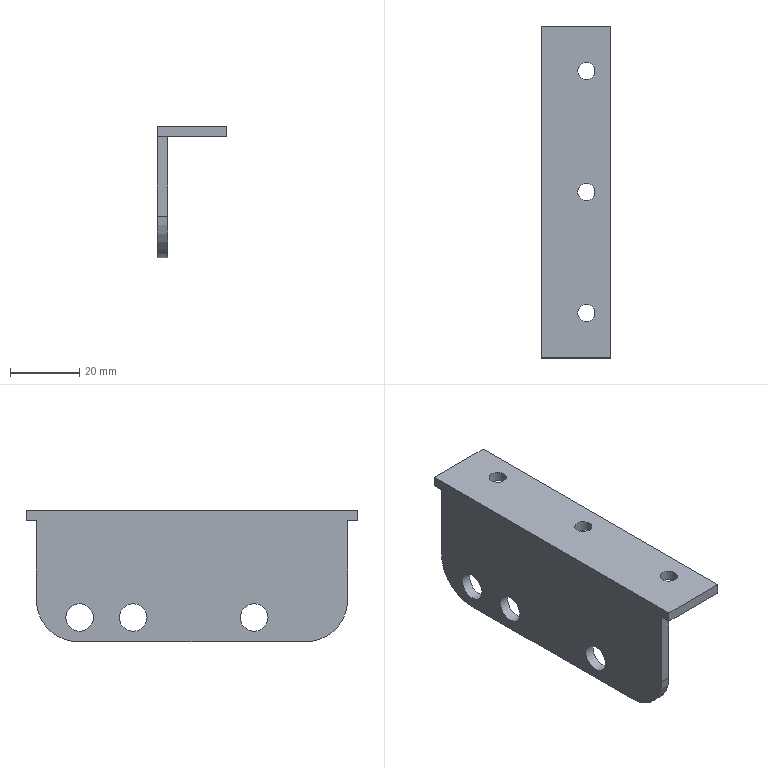Part | STEP file | 1-43.8 | 1 solid | 18 faces | box 20 x 96 x 38 mm | volume 14395 mm3 | plane 10 | cylinder 8 | commonest cylinder face diameters 5 x3 8 x3 24 x2
STEP:
#1=CARTESIAN_POINT('',(0.,0.,0.));
#2=DIRECTION('',(0.,0.,1.));
#3=DIRECTION('',(1.,0.,0.));
#4=AXIS2_PLACEMENT_3D('',#1,#2,#3);
#5=CARTESIAN_POINT('',(10.,-48.,3.));
#6=VERTEX_POINT('',#5);
#7=CARTESIAN_POINT('',(10.,48.,3.));
#8=VERTEX_POINT('',#7);
#9=CARTESIAN_POINT('',(10.,-48.,3.));
#10=DIRECTION('',(0.,1.,0.));
#11=VECTOR('',#10,1.);
#12=LINE('',#9,#11);
#13=CARTESIAN_POINT('',(-38.,0.,3.));
#14=DIRECTION('',(0.,0.,1.));
#15=DIRECTION('',(0.,1.,0.));
#16=AXIS2_PLACEMENT_3D('',#13,#14,#15);
#17=PLANE('',#16);
#18=CARTESIAN_POINT('',(-48.,-48.));
#19=DIRECTION('',(1.,0.));
#20=VECTOR('',#19,1.);
#21=LINE('',#18,#20);
#22=(GEOMETRIC_REPRESENTATION_CONTEXT(2)PARAMETRIC_REPRESENTATION_CONTEXT()REPRESENTATION_CONTEXT('',''));
#23=DEFINITIONAL_REPRESENTATION('',(#21),#22);
#24=PCURVE('',#17,#23);
#25=CARTESIAN_POINT('',(10.,0.,1.5));
#26=DIRECTION('',(1.,0.,0.));
#27=DIRECTION('',(0.,1.,0.));
#28=AXIS2_PLACEMENT_3D('',#25,#26,#27);
#29=PLANE('',#28);
#30=CARTESIAN_POINT('',(-48.,1.5));
#31=DIRECTION('',(1.,0.));
#32=VECTOR('',#31,1.);
#33=LINE('',#30,#32);
#34=(GEOMETRIC_REPRESENTATION_CONTEXT(2)PARAMETRIC_REPRESENTATION_CONTEXT()REPRESENTATION_CONTEXT('',''));
#35=DEFINITIONAL_REPRESENTATION('',(#33),#34);
#36=PCURVE('',#29,#35);
#37=SURFACE_CURVE('',#12,(#24,#36),.PCURVE_S1.);
#38=EDGE_CURVE('',#6,#8,#37,.T.);
#39=ORIENTED_EDGE('',*,*,#38,.T.);
#40=CARTESIAN_POINT('',(-10.,48.,3.));
#41=VERTEX_POINT('',#40);
#42=CARTESIAN_POINT('',(10.,48.,3.));
#43=DIRECTION('',(-1.,0.,0.));
#44=VECTOR('',#43,1.);
#45=LINE('',#42,#44);
#46=CARTESIAN_POINT('',(48.,-48.));
#47=DIRECTION('',(0.,1.));
#48=VECTOR('',#47,1.);
#49=LINE('',#46,#48);
#50=(GEOMETRIC_REPRESENTATION_CONTEXT(2)PARAMETRIC_REPRESENTATION_CONTEXT()REPRESENTATION_CONTEXT('',''));
#51=DEFINITIONAL_REPRESENTATION('',(#49),#50);
#52=PCURVE('',#17,#51);
#53=CARTESIAN_POINT('',(0.,48.,1.5));
#54=DIRECTION('',(0.,1.,0.));
#55=DIRECTION('',(-1.,0.,0.));
#56=AXIS2_PLACEMENT_3D('',#53,#54,#55);
#57=PLANE('',#56);
#58=CARTESIAN_POINT('',(-10.,1.5));
#59=DIRECTION('',(1.,0.));
#60=VECTOR('',#59,1.);
#61=LINE('',#58,#60);
#62=(GEOMETRIC_REPRESENTATION_CONTEXT(2)PARAMETRIC_REPRESENTATION_CONTEXT()REPRESENTATION_CONTEXT('',''));
#63=DEFINITIONAL_REPRESENTATION('',(#61),#62);
#64=PCURVE('',#57,#63);
#65=SURFACE_CURVE('',#45,(#52,#64),.PCURVE_S1.);
#66=EDGE_CURVE('',#8,#41,#65,.T.);
#67=ORIENTED_EDGE('',*,*,#66,.T.);
#68=CARTESIAN_POINT('',(-10.,-48.,3.));
#69=VERTEX_POINT('',#68);
#70=CARTESIAN_POINT('',(-10.,48.,3.));
#71=DIRECTION('',(0.,-1.,0.));
#72=VECTOR('',#71,1.);
#73=LINE('',#70,#72);
#74=CARTESIAN_POINT('',(48.,-28.));
#75=DIRECTION('',(-1.,0.));
#76=VECTOR('',#75,1.);
#77=LINE('',#74,#76);
#78=(GEOMETRIC_REPRESENTATION_CONTEXT(2)PARAMETRIC_REPRESENTATION_CONTEXT()REPRESENTATION_CONTEXT('',''));
#79=DEFINITIONAL_REPRESENTATION('',(#77),#78);
#80=PCURVE('',#17,#79);
#81=CARTESIAN_POINT('',(-10.,0.,10.));
#82=DIRECTION('',(-1.,0.,0.));
#83=DIRECTION('',(0.,-1.,0.));
#84=AXIS2_PLACEMENT_3D('',#81,#82,#83);
#85=PLANE('',#84);
#86=CARTESIAN_POINT('',(-48.,-7.));
#87=DIRECTION('',(1.,0.));
#88=VECTOR('',#87,1.);
#89=LINE('',#86,#88);
#90=(GEOMETRIC_REPRESENTATION_CONTEXT(2)PARAMETRIC_REPRESENTATION_CONTEXT()REPRESENTATION_CONTEXT('',''));
#91=DEFINITIONAL_REPRESENTATION('',(#89),#90);
#92=PCURVE('',#85,#91);
#93=SURFACE_CURVE('',#73,(#80,#92),.PCURVE_S1.);
#94=EDGE_CURVE('',#41,#69,#93,.T.);
#95=ORIENTED_EDGE('',*,*,#94,.T.);
#96=CARTESIAN_POINT('',(-10.,-48.,3.));
#97=DIRECTION('',(1.,0.,0.));
#98=VECTOR('',#97,1.);
#99=LINE('',#96,#98);
#100=CARTESIAN_POINT('',(-48.,-28.));
#101=DIRECTION('',(0.,-1.));
#102=VECTOR('',#101,1.);
#103=LINE('',#100,#102);
#104=(GEOMETRIC_REPRESENTATION_CONTEXT(2)PARAMETRIC_REPRESENTATION_CONTEXT()REPRESENTATION_CONTEXT('',''));
#105=DEFINITIONAL_REPRESENTATION('',(#103),#104);
#106=PCURVE('',#17,#105);
#107=CARTESIAN_POINT('',(0.,-48.,1.5));
#108=DIRECTION('',(0.,-1.,0.));
#109=DIRECTION('',(1.,0.,0.));
#110=AXIS2_PLACEMENT_3D('',#107,#108,#109);
#111=PLANE('',#110);
#112=CARTESIAN_POINT('',(-10.,1.5));
#113=DIRECTION('',(1.,0.));
#114=VECTOR('',#113,1.);
#115=LINE('',#112,#114);
#116=(GEOMETRIC_REPRESENTATION_CONTEXT(2)PARAMETRIC_REPRESENTATION_CONTEXT()REPRESENTATION_CONTEXT('',''));
#117=DEFINITIONAL_REPRESENTATION('',(#115),#116);
#118=PCURVE('',#111,#117);
#119=SURFACE_CURVE('',#99,(#106,#118),.PCURVE_S1.);
#120=EDGE_CURVE('',#69,#6,#119,.T.);
#121=ORIENTED_EDGE('',*,*,#120,.T.);
#122=EDGE_LOOP('',(#39,#67,#95,#121));
#123=FACE_BOUND('',#122,.T.);
#124=CARTESIAN_POINT('',(3.,2.5,3.));
#125=VERTEX_POINT('',#124);
#126=CARTESIAN_POINT('',(3.,0.,3.));
#127=DIRECTION('',(0.,0.,-1.));
#128=DIRECTION('',(0.,1.,0.));
#129=AXIS2_PLACEMENT_3D('',#126,#127,#128);
#130=CIRCLE('',#129,2.5);
#131=CARTESIAN_POINT('',(2.5,-41.));
#132=CARTESIAN_POINT('',(2.5,-45.33));
#133=CARTESIAN_POINT('',(-1.25,-43.165));
#134=CARTESIAN_POINT('',(-5.,-41.));
#135=CARTESIAN_POINT('',(-1.25,-38.835));
#136=CARTESIAN_POINT('',(2.5,-36.67));
#137=CARTESIAN_POINT('',(2.5,-41.));
#138=(BOUNDED_CURVE()B_SPLINE_CURVE(2,(#131,#132,#133,#134,#135,#136,#137),.UNSPECIFIED.,.T.,.F.)B_SPLINE_CURVE_WITH_KNOTS((1,2,2,2,2,1),(-2.094,0.,2.094,4.189,6.283,8.378),.UNSPECIFIED.)CURVE()GEOMETRIC_REPRESENTATION_ITEM()RATIONAL_B_SPLINE_CURVE((1.,0.5,1.,0.5,1.,0.5,1.))REPRESENTATION_ITEM(''));
#139=(GEOMETRIC_REPRESENTATION_CONTEXT(2)PARAMETRIC_REPRESENTATION_CONTEXT()REPRESENTATION_CONTEXT('',''));
#140=DEFINITIONAL_REPRESENTATION('',(#138),#139);
#141=PCURVE('',#17,#140);
#142=CARTESIAN_POINT('',(3.,0.,0.));
#143=DIRECTION('',(0.,0.,1.));
#144=DIRECTION('',(0.,1.,0.));
#145=AXIS2_PLACEMENT_3D('',#142,#143,#144);
#146=CYLINDRICAL_SURFACE('',#145,2.5);
#147=CARTESIAN_POINT('',(6.283,3.));
#148=DIRECTION('',(-1.,0.));
#149=VECTOR('',#148,1.);
#150=LINE('',#147,#149);
#151=(GEOMETRIC_REPRESENTATION_CONTEXT(2)PARAMETRIC_REPRESENTATION_CONTEXT()REPRESENTATION_CONTEXT('',''));
#152=DEFINITIONAL_REPRESENTATION('',(#150),#151);
#153=PCURVE('',#146,#152);
#154=SURFACE_CURVE('',#130,(#141,#153),.PCURVE_S1.);
#155=EDGE_CURVE('',#125,#125,#154,.T.);
#156=ORIENTED_EDGE('',*,*,#155,.T.);
#157=EDGE_LOOP('',(#156));
#158=FACE_BOUND('',#157,.T.);
#159=CARTESIAN_POINT('',(3.,-32.5,3.));
#160=VERTEX_POINT('',#159);
#161=CARTESIAN_POINT('',(3.,-35.,3.));
#162=DIRECTION('',(0.,0.,-1.));
#163=DIRECTION('',(0.,1.,0.));
#164=AXIS2_PLACEMENT_3D('',#161,#162,#163);
#165=CIRCLE('',#164,2.5);
#166=CARTESIAN_POINT('',(-32.5,-41.));
#167=CARTESIAN_POINT('',(-32.5,-45.33));
#168=CARTESIAN_POINT('',(-36.25,-43.165));
#169=CARTESIAN_POINT('',(-40.,-41.));
#170=CARTESIAN_POINT('',(-36.25,-38.835));
#171=CARTESIAN_POINT('',(-32.5,-36.67));
#172=CARTESIAN_POINT('',(-32.5,-41.));
#173=(BOUNDED_CURVE()B_SPLINE_CURVE(2,(#166,#167,#168,#169,#170,#171,#172),.UNSPECIFIED.,.T.,.F.)B_SPLINE_CURVE_WITH_KNOTS((1,2,2,2,2,1),(-2.094,0.,2.094,4.189,6.283,8.378),.UNSPECIFIED.)CURVE()GEOMETRIC_REPRESENTATION_ITEM()RATIONAL_B_SPLINE_CURVE((1.,0.5,1.,0.5,1.,0.5,1.))REPRESENTATION_ITEM(''));
#174=(GEOMETRIC_REPRESENTATION_CONTEXT(2)PARAMETRIC_REPRESENTATION_CONTEXT()REPRESENTATION_CONTEXT('',''));
#175=DEFINITIONAL_REPRESENTATION('',(#173),#174);
#176=PCURVE('',#17,#175);
#177=CARTESIAN_POINT('',(3.,-35.,0.));
#178=DIRECTION('',(0.,0.,1.));
#179=DIRECTION('',(0.,1.,0.));
#180=AXIS2_PLACEMENT_3D('',#177,#178,#179);
#181=CYLINDRICAL_SURFACE('',#180,2.5);
#182=CARTESIAN_POINT('',(6.283,3.));
#183=DIRECTION('',(-1.,0.));
#184=VECTOR('',#183,1.);
#185=LINE('',#182,#184);
#186=(GEOMETRIC_REPRESENTATION_CONTEXT(2)PARAMETRIC_REPRESENTATION_CONTEXT()REPRESENTATION_CONTEXT('',''));
#187=DEFINITIONAL_REPRESENTATION('',(#185),#186);
#188=PCURVE('',#181,#187);
#189=SURFACE_CURVE('',#165,(#176,#188),.PCURVE_S1.);
#190=EDGE_CURVE('',#160,#160,#189,.T.);
#191=ORIENTED_EDGE('',*,*,#190,.T.);
#192=EDGE_LOOP('',(#191));
#193=FACE_BOUND('',#192,.T.);
#194=CARTESIAN_POINT('',(3.,37.5,3.));
#195=VERTEX_POINT('',#194);
#196=CARTESIAN_POINT('',(3.,35.,3.));
#197=DIRECTION('',(0.,0.,-1.));
#198=DIRECTION('',(0.,1.,0.));
#199=AXIS2_PLACEMENT_3D('',#196,#197,#198);
#200=CIRCLE('',#199,2.5);
#201=CARTESIAN_POINT('',(37.5,-41.));
#202=CARTESIAN_POINT('',(37.5,-45.33));
#203=CARTESIAN_POINT('',(33.75,-43.165));
#204=CARTESIAN_POINT('',(30.,-41.));
#205=CARTESIAN_POINT('',(33.75,-38.835));
#206=CARTESIAN_POINT('',(37.5,-36.67));
#207=CARTESIAN_POINT('',(37.5,-41.));
#208=(BOUNDED_CURVE()B_SPLINE_CURVE(2,(#201,#202,#203,#204,#205,#206,#207),.UNSPECIFIED.,.T.,.F.)B_SPLINE_CURVE_WITH_KNOTS((1,2,2,2,2,1),(-2.094,0.,2.094,4.189,6.283,8.378),.UNSPECIFIED.)CURVE()GEOMETRIC_REPRESENTATION_ITEM()RATIONAL_B_SPLINE_CURVE((1.,0.5,1.,0.5,1.,0.5,1.))REPRESENTATION_ITEM(''));
#209=(GEOMETRIC_REPRESENTATION_CONTEXT(2)PARAMETRIC_REPRESENTATION_CONTEXT()REPRESENTATION_CONTEXT('',''));
#210=DEFINITIONAL_REPRESENTATION('',(#208),#209);
#211=PCURVE('',#17,#210);
#212=CARTESIAN_POINT('',(3.,35.,0.));
#213=DIRECTION('',(0.,0.,1.));
#214=DIRECTION('',(0.,1.,0.));
#215=AXIS2_PLACEMENT_3D('',#212,#213,#214);
#216=CYLINDRICAL_SURFACE('',#215,2.5);
#217=CARTESIAN_POINT('',(6.283,3.));
#218=DIRECTION('',(-1.,0.));
#219=VECTOR('',#218,1.);
#220=LINE('',#217,#219);
#221=(GEOMETRIC_REPRESENTATION_CONTEXT(2)PARAMETRIC_REPRESENTATION_CONTEXT()REPRESENTATION_CONTEXT('',''));
#222=DEFINITIONAL_REPRESENTATION('',(#220),#221);
#223=PCURVE('',#216,#222);
#224=SURFACE_CURVE('',#200,(#211,#223),.PCURVE_S1.);
#225=EDGE_CURVE('',#195,#195,#224,.T.);
#226=ORIENTED_EDGE('',*,*,#225,.T.);
#227=EDGE_LOOP('',(#226));
#228=FACE_BOUND('',#227,.T.);
#229=ADVANCED_FACE('',(#123,#158,#193,#228),#17,.T.);
#230=CARTESIAN_POINT('',(10.,-48.,0.));
#231=VERTEX_POINT('',#230);
#232=CARTESIAN_POINT('',(10.,48.,0.));
#233=VERTEX_POINT('',#232);
#234=CARTESIAN_POINT('',(10.,-48.,0.));
#235=DIRECTION('',(0.,1.,0.));
#236=VECTOR('',#235,1.);
#237=LINE('',#234,#236);
#238=CARTESIAN_POINT('',(-48.,-1.5));
#239=DIRECTION('',(1.,0.));
#240=VECTOR('',#239,1.);
#241=LINE('',#238,#240);
#242=(GEOMETRIC_REPRESENTATION_CONTEXT(2)PARAMETRIC_REPRESENTATION_CONTEXT()REPRESENTATION_CONTEXT('',''));
#243=DEFINITIONAL_REPRESENTATION('',(#241),#242);
#244=PCURVE('',#29,#243);
#245=CARTESIAN_POINT('',(-38.,0.,0.));
#246=DIRECTION('',(0.,0.,1.));
#247=DIRECTION('',(0.,1.,0.));
#248=AXIS2_PLACEMENT_3D('',#245,#246,#247);
#249=PLANE('',#248);
#250=CARTESIAN_POINT('',(-48.,-48.));
#251=DIRECTION('',(1.,0.));
#252=VECTOR('',#251,1.);
#253=LINE('',#250,#252);
#254=(GEOMETRIC_REPRESENTATION_CONTEXT(2)PARAMETRIC_REPRESENTATION_CONTEXT()REPRESENTATION_CONTEXT('',''));
#255=DEFINITIONAL_REPRESENTATION('',(#253),#254);
#256=PCURVE('',#249,#255);
#257=SURFACE_CURVE('',#237,(#244,#256),.PCURVE_S1.);
#258=EDGE_CURVE('',#231,#233,#257,.T.);
#259=ORIENTED_EDGE('',*,*,#258,.T.);
#260=CARTESIAN_POINT('',(10.,48.,0.));
#261=DIRECTION('',(0.,0.,1.));
#262=VECTOR('',#261,1.);
#263=LINE('',#260,#262);
#264=CARTESIAN_POINT('',(48.,-1.5));
#265=DIRECTION('',(0.,1.));
#266=VECTOR('',#265,1.);
#267=LINE('',#264,#266);
#268=(GEOMETRIC_REPRESENTATION_CONTEXT(2)PARAMETRIC_REPRESENTATION_CONTEXT()REPRESENTATION_CONTEXT('',''));
#269=DEFINITIONAL_REPRESENTATION('',(#267),#268);
#270=PCURVE('',#29,#269);
#271=CARTESIAN_POINT('',(-10.,-1.5));
#272=DIRECTION('',(0.,1.));
#273=VECTOR('',#272,1.);
#274=LINE('',#271,#273);
#275=(GEOMETRIC_REPRESENTATION_CONTEXT(2)PARAMETRIC_REPRESENTATION_CONTEXT()REPRESENTATION_CONTEXT('',''));
#276=DEFINITIONAL_REPRESENTATION('',(#274),#275);
#277=PCURVE('',#57,#276);
#278=SURFACE_CURVE('',#263,(#270,#277),.PCURVE_S1.);
#279=EDGE_CURVE('',#233,#8,#278,.T.);
#280=ORIENTED_EDGE('',*,*,#279,.T.);
#281=ORIENTED_EDGE('',*,*,#38,.F.);
#282=CARTESIAN_POINT('',(10.,-48.,0.));
#283=DIRECTION('',(0.,0.,1.));
#284=VECTOR('',#283,1.);
#285=LINE('',#282,#284);
#286=CARTESIAN_POINT('',(-48.,-1.5));
#287=DIRECTION('',(0.,1.));
#288=VECTOR('',#287,1.);
#289=LINE('',#286,#288);
#290=(GEOMETRIC_REPRESENTATION_CONTEXT(2)PARAMETRIC_REPRESENTATION_CONTEXT()REPRESENTATION_CONTEXT('',''));
#291=DEFINITIONAL_REPRESENTATION('',(#289),#290);
#292=PCURVE('',#29,#291);
#293=CARTESIAN_POINT('',(10.,-1.5));
#294=DIRECTION('',(0.,1.));
#295=VECTOR('',#294,1.);
#296=LINE('',#293,#295);
#297=(GEOMETRIC_REPRESENTATION_CONTEXT(2)PARAMETRIC_REPRESENTATION_CONTEXT()REPRESENTATION_CONTEXT('',''));
#298=DEFINITIONAL_REPRESENTATION('',(#296),#297);
#299=PCURVE('',#111,#298);
#300=SURFACE_CURVE('',#285,(#292,#299),.PCURVE_S1.);
#301=EDGE_CURVE('',#231,#6,#300,.T.);
#302=ORIENTED_EDGE('',*,*,#301,.F.);
#303=EDGE_LOOP('',(#259,#280,#281,#302));
#304=FACE_BOUND('',#303,.T.);
#305=ADVANCED_FACE('',(#304),#29,.T.);
#306=CARTESIAN_POINT('',(-10.,48.,0.));
#307=VERTEX_POINT('',#306);
#308=CARTESIAN_POINT('',(10.,48.,0.));
#309=DIRECTION('',(-1.,0.,0.));
#310=VECTOR('',#309,1.);
#311=LINE('',#308,#310);
#312=CARTESIAN_POINT('',(-10.,-1.5));
#313=DIRECTION('',(1.,0.));
#314=VECTOR('',#313,1.);
#315=LINE('',#312,#314);
#316=(GEOMETRIC_REPRESENTATION_CONTEXT(2)PARAMETRIC_REPRESENTATION_CONTEXT()REPRESENTATION_CONTEXT('',''));
#317=DEFINITIONAL_REPRESENTATION('',(#315),#316);
#318=PCURVE('',#57,#317);
#319=CARTESIAN_POINT('',(48.,-48.));
#320=DIRECTION('',(0.,1.));
#321=VECTOR('',#320,1.);
#322=LINE('',#319,#321);
#323=(GEOMETRIC_REPRESENTATION_CONTEXT(2)PARAMETRIC_REPRESENTATION_CONTEXT()REPRESENTATION_CONTEXT('',''));
#324=DEFINITIONAL_REPRESENTATION('',(#322),#323);
#325=PCURVE('',#249,#324);
#326=SURFACE_CURVE('',#311,(#318,#325),.PCURVE_S1.);
#327=EDGE_CURVE('',#233,#307,#326,.T.);
#328=ORIENTED_EDGE('',*,*,#327,.T.);
#329=CARTESIAN_POINT('',(-10.,48.,0.));
#330=DIRECTION('',(0.,0.,1.));
#331=VECTOR('',#330,1.);
#332=LINE('',#329,#331);
#333=CARTESIAN_POINT('',(10.,-1.5));
#334=DIRECTION('',(0.,1.));
#335=VECTOR('',#334,1.);
#336=LINE('',#333,#335);
#337=(GEOMETRIC_REPRESENTATION_CONTEXT(2)PARAMETRIC_REPRESENTATION_CONTEXT()REPRESENTATION_CONTEXT('',''));
#338=DEFINITIONAL_REPRESENTATION('',(#336),#337);
#339=PCURVE('',#57,#338);
#340=CARTESIAN_POINT('',(-48.,-10.));
#341=DIRECTION('',(0.,1.));
#342=VECTOR('',#341,1.);
#343=LINE('',#340,#342);
#344=(GEOMETRIC_REPRESENTATION_CONTEXT(2)PARAMETRIC_REPRESENTATION_CONTEXT()REPRESENTATION_CONTEXT('',''));
#345=DEFINITIONAL_REPRESENTATION('',(#343),#344);
#346=PCURVE('',#85,#345);
#347=SURFACE_CURVE('',#332,(#339,#346),.PCURVE_S1.);
#348=EDGE_CURVE('',#307,#41,#347,.T.);
#349=ORIENTED_EDGE('',*,*,#348,.T.);
#350=ORIENTED_EDGE('',*,*,#66,.F.);
#351=ORIENTED_EDGE('',*,*,#279,.F.);
#352=EDGE_LOOP('',(#328,#349,#350,#351));
#353=FACE_BOUND('',#352,.T.);
#354=ADVANCED_FACE('',(#353),#57,.T.);
#355=CARTESIAN_POINT('',(-10.,-48.,0.));
#356=VERTEX_POINT('',#355);
#357=CARTESIAN_POINT('',(-10.,-48.,0.));
#358=DIRECTION('',(1.,0.,0.));
#359=VECTOR('',#358,1.);
#360=LINE('',#357,#359);
#361=CARTESIAN_POINT('',(-10.,-1.5));
#362=DIRECTION('',(1.,0.));
#363=VECTOR('',#362,1.);
#364=LINE('',#361,#363);
#365=(GEOMETRIC_REPRESENTATION_CONTEXT(2)PARAMETRIC_REPRESENTATION_CONTEXT()REPRESENTATION_CONTEXT('',''));
#366=DEFINITIONAL_REPRESENTATION('',(#364),#365);
#367=PCURVE('',#111,#366);
#368=CARTESIAN_POINT('',(-48.,-28.));
#369=DIRECTION('',(0.,-1.));
#370=VECTOR('',#369,1.);
#371=LINE('',#368,#370);
#372=(GEOMETRIC_REPRESENTATION_CONTEXT(2)PARAMETRIC_REPRESENTATION_CONTEXT()REPRESENTATION_CONTEXT('',''));
#373=DEFINITIONAL_REPRESENTATION('',(#371),#372);
#374=PCURVE('',#249,#373);
#375=SURFACE_CURVE('',#360,(#367,#374),.PCURVE_S1.);
#376=EDGE_CURVE('',#356,#231,#375,.T.);
#377=ORIENTED_EDGE('',*,*,#376,.T.);
#378=ORIENTED_EDGE('',*,*,#301,.T.);
#379=ORIENTED_EDGE('',*,*,#120,.F.);
#380=CARTESIAN_POINT('',(-10.,-48.,0.));
#381=DIRECTION('',(0.,0.,1.));
#382=VECTOR('',#381,1.);
#383=LINE('',#380,#382);
#384=CARTESIAN_POINT('',(-10.,-1.5));
#385=DIRECTION('',(0.,1.));
#386=VECTOR('',#385,1.);
#387=LINE('',#384,#386);
#388=(GEOMETRIC_REPRESENTATION_CONTEXT(2)PARAMETRIC_REPRESENTATION_CONTEXT()REPRESENTATION_CONTEXT('',''));
#389=DEFINITIONAL_REPRESENTATION('',(#387),#388);
#390=PCURVE('',#111,#389);
#391=CARTESIAN_POINT('',(48.,-10.));
#392=DIRECTION('',(0.,1.));
#393=VECTOR('',#392,1.);
#394=LINE('',#391,#393);
#395=(GEOMETRIC_REPRESENTATION_CONTEXT(2)PARAMETRIC_REPRESENTATION_CONTEXT()REPRESENTATION_CONTEXT('',''));
#396=DEFINITIONAL_REPRESENTATION('',(#394),#395);
#397=PCURVE('',#85,#396);
#398=SURFACE_CURVE('',#383,(#390,#397),.PCURVE_S1.);
#399=EDGE_CURVE('',#356,#69,#398,.T.);
#400=ORIENTED_EDGE('',*,*,#399,.F.);
#401=EDGE_LOOP('',(#377,#378,#379,#400));
#402=FACE_BOUND('',#401,.T.);
#403=ADVANCED_FACE('',(#402),#111,.T.);
#404=CARTESIAN_POINT('',(3.,2.5,0.));
#405=VERTEX_POINT('',#404);
#406=CARTESIAN_POINT('',(3.,2.5,0.));
#407=DIRECTION('',(0.,0.,1.));
#408=VECTOR('',#407,1.);
#409=LINE('',#406,#408);
#410=CARTESIAN_POINT('',(6.283,0.));
#411=DIRECTION('',(0.,1.));
#412=VECTOR('',#411,1.);
#413=LINE('',#410,#412);
#414=(GEOMETRIC_REPRESENTATION_CONTEXT(2)PARAMETRIC_REPRESENTATION_CONTEXT()REPRESENTATION_CONTEXT('',''));
#415=DEFINITIONAL_REPRESENTATION('',(#413),#414);
#416=PCURVE('',#146,#415);
#417=CARTESIAN_POINT('',(0.,0.));
#418=DIRECTION('',(0.,1.));
#419=VECTOR('',#418,1.);
#420=LINE('',#417,#419);
#421=(GEOMETRIC_REPRESENTATION_CONTEXT(2)PARAMETRIC_REPRESENTATION_CONTEXT()REPRESENTATION_CONTEXT('',''));
#422=DEFINITIONAL_REPRESENTATION('',(#420),#421);
#423=PCURVE('',#146,#422);
#424=SEAM_CURVE('',#409,(#416,#423),.PCURVE_S1.);
#425=EDGE_CURVE('',#405,#125,#424,.T.);
#426=ORIENTED_EDGE('',*,*,#425,.T.);
#427=ORIENTED_EDGE('',*,*,#155,.T.);
#428=ORIENTED_EDGE('',*,*,#425,.F.);
#429=CARTESIAN_POINT('',(3.,0.,0.));
#430=DIRECTION('',(0.,0.,-1.));
#431=DIRECTION('',(0.,1.,0.));
#432=AXIS2_PLACEMENT_3D('',#429,#430,#431);
#433=CIRCLE('',#432,2.5);
#434=CARTESIAN_POINT('',(6.283,0.));
#435=DIRECTION('',(-1.,0.));
#436=VECTOR('',#435,1.);
#437=LINE('',#434,#436);
#438=(GEOMETRIC_REPRESENTATION_CONTEXT(2)PARAMETRIC_REPRESENTATION_CONTEXT()REPRESENTATION_CONTEXT('',''));
#439=DEFINITIONAL_REPRESENTATION('',(#437),#438);
#440=PCURVE('',#146,#439);
#441=CARTESIAN_POINT('',(2.5,-41.));
#442=CARTESIAN_POINT('',(2.5,-45.33));
#443=CARTESIAN_POINT('',(-1.25,-43.165));
#444=CARTESIAN_POINT('',(-5.,-41.));
#445=CARTESIAN_POINT('',(-1.25,-38.835));
#446=CARTESIAN_POINT('',(2.5,-36.67));
#447=CARTESIAN_POINT('',(2.5,-41.));
#448=(BOUNDED_CURVE()B_SPLINE_CURVE(2,(#441,#442,#443,#444,#445,#446,#447),.UNSPECIFIED.,.T.,.F.)B_SPLINE_CURVE_WITH_KNOTS((1,2,2,2,2,1),(-2.094,0.,2.094,4.189,6.283,8.378),.UNSPECIFIED.)CURVE()GEOMETRIC_REPRESENTATION_ITEM()RATIONAL_B_SPLINE_CURVE((1.,0.5,1.,0.5,1.,0.5,1.))REPRESENTATION_ITEM(''));
#449=(GEOMETRIC_REPRESENTATION_CONTEXT(2)PARAMETRIC_REPRESENTATION_CONTEXT()REPRESENTATION_CONTEXT('',''));
#450=DEFINITIONAL_REPRESENTATION('',(#448),#449);
#451=PCURVE('',#249,#450);
#452=SURFACE_CURVE('',#433,(#440,#451),.PCURVE_S1.);
#453=EDGE_CURVE('',#405,#405,#452,.T.);
#454=ORIENTED_EDGE('',*,*,#453,.F.);
#455=EDGE_LOOP('',(#426,#427,#428,#454));
#456=FACE_BOUND('',#455,.F.);
#457=ADVANCED_FACE('',(#456),#146,.F.);
#458=CARTESIAN_POINT('',(3.,-32.5,0.));
#459=VERTEX_POINT('',#458);
#460=CARTESIAN_POINT('',(3.,-32.5,0.));
#461=DIRECTION('',(0.,0.,1.));
#462=VECTOR('',#461,1.);
#463=LINE('',#460,#462);
#464=CARTESIAN_POINT('',(6.283,0.));
#465=DIRECTION('',(0.,1.));
#466=VECTOR('',#465,1.);
#467=LINE('',#464,#466);
#468=(GEOMETRIC_REPRESENTATION_CONTEXT(2)PARAMETRIC_REPRESENTATION_CONTEXT()REPRESENTATION_CONTEXT('',''));
#469=DEFINITIONAL_REPRESENTATION('',(#467),#468);
#470=PCURVE('',#181,#469);
#471=CARTESIAN_POINT('',(0.,0.));
#472=DIRECTION('',(0.,1.));
#473=VECTOR('',#472,1.);
#474=LINE('',#471,#473);
#475=(GEOMETRIC_REPRESENTATION_CONTEXT(2)PARAMETRIC_REPRESENTATION_CONTEXT()REPRESENTATION_CONTEXT('',''));
#476=DEFINITIONAL_REPRESENTATION('',(#474),#475);
#477=PCURVE('',#181,#476);
#478=SEAM_CURVE('',#463,(#470,#477),.PCURVE_S1.);
#479=EDGE_CURVE('',#459,#160,#478,.T.);
#480=ORIENTED_EDGE('',*,*,#479,.T.);
#481=ORIENTED_EDGE('',*,*,#190,.T.);
#482=ORIENTED_EDGE('',*,*,#479,.F.);
#483=CARTESIAN_POINT('',(3.,-35.,0.));
#484=DIRECTION('',(0.,0.,-1.));
#485=DIRECTION('',(0.,1.,0.));
#486=AXIS2_PLACEMENT_3D('',#483,#484,#485);
#487=CIRCLE('',#486,2.5);
#488=CARTESIAN_POINT('',(6.283,0.));
#489=DIRECTION('',(-1.,0.));
#490=VECTOR('',#489,1.);
#491=LINE('',#488,#490);
#492=(GEOMETRIC_REPRESENTATION_CONTEXT(2)PARAMETRIC_REPRESENTATION_CONTEXT()REPRESENTATION_CONTEXT('',''));
#493=DEFINITIONAL_REPRESENTATION('',(#491),#492);
#494=PCURVE('',#181,#493);
#495=CARTESIAN_POINT('',(-32.5,-41.));
#496=CARTESIAN_POINT('',(-32.5,-45.33));
#497=CARTESIAN_POINT('',(-36.25,-43.165));
#498=CARTESIAN_POINT('',(-40.,-41.));
#499=CARTESIAN_POINT('',(-36.25,-38.835));
#500=CARTESIAN_POINT('',(-32.5,-36.67));
#501=CARTESIAN_POINT('',(-32.5,-41.));
#502=(BOUNDED_CURVE()B_SPLINE_CURVE(2,(#495,#496,#497,#498,#499,#500,#501),.UNSPECIFIED.,.T.,.F.)B_SPLINE_CURVE_WITH_KNOTS((1,2,2,2,2,1),(-2.094,0.,2.094,4.189,6.283,8.378),.UNSPECIFIED.)CURVE()GEOMETRIC_REPRESENTATION_ITEM()RATIONAL_B_SPLINE_CURVE((1.,0.5,1.,0.5,1.,0.5,1.))REPRESENTATION_ITEM(''));
#503=(GEOMETRIC_REPRESENTATION_CONTEXT(2)PARAMETRIC_REPRESENTATION_CONTEXT()REPRESENTATION_CONTEXT('',''));
#504=DEFINITIONAL_REPRESENTATION('',(#502),#503);
#505=PCURVE('',#249,#504);
#506=SURFACE_CURVE('',#487,(#494,#505),.PCURVE_S1.);
#507=EDGE_CURVE('',#459,#459,#506,.T.);
#508=ORIENTED_EDGE('',*,*,#507,.F.);
#509=EDGE_LOOP('',(#480,#481,#482,#508));
#510=FACE_BOUND('',#509,.F.);
#511=ADVANCED_FACE('',(#510),#181,.F.);
#512=CARTESIAN_POINT('',(3.,37.5,0.));
#513=VERTEX_POINT('',#512);
#514=CARTESIAN_POINT('',(3.,37.5,0.));
#515=DIRECTION('',(0.,0.,1.));
#516=VECTOR('',#515,1.);
#517=LINE('',#514,#516);
#518=CARTESIAN_POINT('',(6.283,0.));
#519=DIRECTION('',(0.,1.));
#520=VECTOR('',#519,1.);
#521=LINE('',#518,#520);
#522=(GEOMETRIC_REPRESENTATION_CONTEXT(2)PARAMETRIC_REPRESENTATION_CONTEXT()REPRESENTATION_CONTEXT('',''));
#523=DEFINITIONAL_REPRESENTATION('',(#521),#522);
#524=PCURVE('',#216,#523);
#525=CARTESIAN_POINT('',(0.,0.));
#526=DIRECTION('',(0.,1.));
#527=VECTOR('',#526,1.);
#528=LINE('',#525,#527);
#529=(GEOMETRIC_REPRESENTATION_CONTEXT(2)PARAMETRIC_REPRESENTATION_CONTEXT()REPRESENTATION_CONTEXT('',''));
#530=DEFINITIONAL_REPRESENTATION('',(#528),#529);
#531=PCURVE('',#216,#530);
#532=SEAM_CURVE('',#517,(#524,#531),.PCURVE_S1.);
#533=EDGE_CURVE('',#513,#195,#532,.T.);
#534=ORIENTED_EDGE('',*,*,#533,.T.);
#535=ORIENTED_EDGE('',*,*,#225,.T.);
#536=ORIENTED_EDGE('',*,*,#533,.F.);
#537=CARTESIAN_POINT('',(3.,35.,0.));
#538=DIRECTION('',(0.,0.,-1.));
#539=DIRECTION('',(0.,1.,0.));
#540=AXIS2_PLACEMENT_3D('',#537,#538,#539);
#541=CIRCLE('',#540,2.5);
#542=CARTESIAN_POINT('',(6.283,0.));
#543=DIRECTION('',(-1.,0.));
#544=VECTOR('',#543,1.);
#545=LINE('',#542,#544);
#546=(GEOMETRIC_REPRESENTATION_CONTEXT(2)PARAMETRIC_REPRESENTATION_CONTEXT()REPRESENTATION_CONTEXT('',''));
#547=DEFINITIONAL_REPRESENTATION('',(#545),#546);
#548=PCURVE('',#216,#547);
#549=CARTESIAN_POINT('',(37.5,-41.));
#550=CARTESIAN_POINT('',(37.5,-45.33));
#551=CARTESIAN_POINT('',(33.75,-43.165));
#552=CARTESIAN_POINT('',(30.,-41.));
#553=CARTESIAN_POINT('',(33.75,-38.835));
#554=CARTESIAN_POINT('',(37.5,-36.67));
#555=CARTESIAN_POINT('',(37.5,-41.));
#556=(BOUNDED_CURVE()B_SPLINE_CURVE(2,(#549,#550,#551,#552,#553,#554,#555),.UNSPECIFIED.,.T.,.F.)B_SPLINE_CURVE_WITH_KNOTS((1,2,2,2,2,1),(-2.094,0.,2.094,4.189,6.283,8.378),.UNSPECIFIED.)CURVE()GEOMETRIC_REPRESENTATION_ITEM()RATIONAL_B_SPLINE_CURVE((1.,0.5,1.,0.5,1.,0.5,1.))REPRESENTATION_ITEM(''));
#557=(GEOMETRIC_REPRESENTATION_CONTEXT(2)PARAMETRIC_REPRESENTATION_CONTEXT()REPRESENTATION_CONTEXT('',''));
#558=DEFINITIONAL_REPRESENTATION('',(#556),#557);
#559=PCURVE('',#249,#558);
#560=SURFACE_CURVE('',#541,(#548,#559),.PCURVE_S1.);
#561=EDGE_CURVE('',#513,#513,#560,.T.);
#562=ORIENTED_EDGE('',*,*,#561,.F.);
#563=EDGE_LOOP('',(#534,#535,#536,#562));
#564=FACE_BOUND('',#563,.F.);
#565=ADVANCED_FACE('',(#564),#216,.F.);
#566=ORIENTED_EDGE('',*,*,#258,.T.);
#567=ORIENTED_EDGE('',*,*,#327,.T.);
#568=CARTESIAN_POINT('',(-10.,45.,0.));
#569=VERTEX_POINT('',#568);
#570=CARTESIAN_POINT('',(-10.,48.,0.));
#571=DIRECTION('',(0.,-1.,0.));
#572=VECTOR('',#571,1.);
#573=LINE('',#570,#572);
#574=CARTESIAN_POINT('',(48.,-28.));
#575=DIRECTION('',(-1.,0.));
#576=VECTOR('',#575,1.);
#577=LINE('',#574,#576);
#578=(GEOMETRIC_REPRESENTATION_CONTEXT(2)PARAMETRIC_REPRESENTATION_CONTEXT()REPRESENTATION_CONTEXT('',''));
#579=DEFINITIONAL_REPRESENTATION('',(#577),#578);
#580=PCURVE('',#249,#579);
#581=CARTESIAN_POINT('',(-48.,-10.));
#582=DIRECTION('',(1.,0.));
#583=VECTOR('',#582,1.);
#584=LINE('',#581,#583);
#585=(GEOMETRIC_REPRESENTATION_CONTEXT(2)PARAMETRIC_REPRESENTATION_CONTEXT()REPRESENTATION_CONTEXT('',''));
#586=DEFINITIONAL_REPRESENTATION('',(#584),#585);
#587=PCURVE('',#85,#586);
#588=SURFACE_CURVE('',#573,(#580,#587),.PCURVE_S1.);
#589=EDGE_CURVE('',#307,#569,#588,.T.);
#590=ORIENTED_EDGE('',*,*,#589,.T.);
#591=CARTESIAN_POINT('',(-7.,45.,0.));
#592=VERTEX_POINT('',#591);
#593=CARTESIAN_POINT('',(-10.,45.,0.));
#594=DIRECTION('',(1.,0.,0.));
#595=VECTOR('',#594,1.);
#596=LINE('',#593,#595);
#597=CARTESIAN_POINT('',(45.,-28.));
#598=DIRECTION('',(0.,-1.));
#599=VECTOR('',#598,1.);
#600=LINE('',#597,#599);
#601=(GEOMETRIC_REPRESENTATION_CONTEXT(2)PARAMETRIC_REPRESENTATION_CONTEXT()REPRESENTATION_CONTEXT('',''));
#602=DEFINITIONAL_REPRESENTATION('',(#600),#601);
#603=PCURVE('',#249,#602);
#604=CARTESIAN_POINT('',(-8.5,45.,-17.5));
#605=DIRECTION('',(0.,-1.,0.));
#606=DIRECTION('',(0.,0.,-1.));
#607=AXIS2_PLACEMENT_3D('',#604,#605,#606);
#608=PLANE('',#607);
#609=CARTESIAN_POINT('',(-17.5,-1.5));
#610=DIRECTION('',(0.,1.));
#611=VECTOR('',#610,1.);
#612=LINE('',#609,#611);
#613=(GEOMETRIC_REPRESENTATION_CONTEXT(2)PARAMETRIC_REPRESENTATION_CONTEXT()REPRESENTATION_CONTEXT('',''));
#614=DEFINITIONAL_REPRESENTATION('',(#612),#613);
#615=PCURVE('',#608,#614);
#616=SURFACE_CURVE('',#596,(#603,#615),.PCURVE_S1.);
#617=EDGE_CURVE('',#569,#592,#616,.T.);
#618=ORIENTED_EDGE('',*,*,#617,.T.);
#619=CARTESIAN_POINT('',(-7.,-45.,0.));
#620=VERTEX_POINT('',#619);
#621=CARTESIAN_POINT('',(-7.,-45.,0.));
#622=DIRECTION('',(0.,1.,0.));
#623=VECTOR('',#622,1.);
#624=LINE('',#621,#623);
#625=CARTESIAN_POINT('',(-45.,-31.));
#626=DIRECTION('',(1.,0.));
#627=VECTOR('',#626,1.);
#628=LINE('',#625,#627);
#629=(GEOMETRIC_REPRESENTATION_CONTEXT(2)PARAMETRIC_REPRESENTATION_CONTEXT()REPRESENTATION_CONTEXT('',''));
#630=DEFINITIONAL_REPRESENTATION('',(#628),#629);
#631=PCURVE('',#249,#630);
#632=CARTESIAN_POINT('',(-7.,0.,10.));
#633=DIRECTION('',(-1.,0.,0.));
#634=DIRECTION('',(0.,-1.,0.));
#635=AXIS2_PLACEMENT_3D('',#632,#633,#634);
#636=PLANE('',#635);
#637=CARTESIAN_POINT('',(45.,-10.));
#638=DIRECTION('',(-1.,0.));
#639=VECTOR('',#638,1.);
#640=LINE('',#637,#639);
#641=(GEOMETRIC_REPRESENTATION_CONTEXT(2)PARAMETRIC_REPRESENTATION_CONTEXT()REPRESENTATION_CONTEXT('',''));
#642=DEFINITIONAL_REPRESENTATION('',(#640),#641);
#643=PCURVE('',#636,#642);
#644=SURFACE_CURVE('',#624,(#631,#643),.PCURVE_S1.);
#645=EDGE_CURVE('',#620,#592,#644,.T.);
#646=ORIENTED_EDGE('',*,*,#645,.F.);
#647=CARTESIAN_POINT('',(-10.,-45.,0.));
#648=VERTEX_POINT('',#647);
#649=CARTESIAN_POINT('',(-10.,-45.,0.));
#650=DIRECTION('',(1.,0.,0.));
#651=VECTOR('',#650,1.);
#652=LINE('',#649,#651);
#653=CARTESIAN_POINT('',(-45.,-28.));
#654=DIRECTION('',(0.,-1.));
#655=VECTOR('',#654,1.);
#656=LINE('',#653,#655);
#657=(GEOMETRIC_REPRESENTATION_CONTEXT(2)PARAMETRIC_REPRESENTATION_CONTEXT()REPRESENTATION_CONTEXT('',''));
#658=DEFINITIONAL_REPRESENTATION('',(#656),#657);
#659=PCURVE('',#249,#658);
#660=CARTESIAN_POINT('',(-8.5,-45.,-17.5));
#661=DIRECTION('',(0.,1.,0.));
#662=DIRECTION('',(0.,0.,1.));
#663=AXIS2_PLACEMENT_3D('',#660,#661,#662);
#664=PLANE('',#663);
#665=CARTESIAN_POINT('',(17.5,-1.5));
#666=DIRECTION('',(0.,1.));
#667=VECTOR('',#666,1.);
#668=LINE('',#665,#667);
#669=(GEOMETRIC_REPRESENTATION_CONTEXT(2)PARAMETRIC_REPRESENTATION_CONTEXT()REPRESENTATION_CONTEXT('',''));
#670=DEFINITIONAL_REPRESENTATION('',(#668),#669);
#671=PCURVE('',#664,#670);
#672=SURFACE_CURVE('',#652,(#659,#671),.PCURVE_S1.);
#673=EDGE_CURVE('',#648,#620,#672,.T.);
#674=ORIENTED_EDGE('',*,*,#673,.F.);
#675=CARTESIAN_POINT('',(-10.,-45.,0.));
#676=DIRECTION('',(0.,-1.,0.));
#677=VECTOR('',#676,1.);
#678=LINE('',#675,#677);
#679=CARTESIAN_POINT('',(-45.,-28.));
#680=DIRECTION('',(-1.,0.));
#681=VECTOR('',#680,1.);
#682=LINE('',#679,#681);
#683=(GEOMETRIC_REPRESENTATION_CONTEXT(2)PARAMETRIC_REPRESENTATION_CONTEXT()REPRESENTATION_CONTEXT('',''));
#684=DEFINITIONAL_REPRESENTATION('',(#682),#683);
#685=PCURVE('',#249,#684);
#686=CARTESIAN_POINT('',(45.,-10.));
#687=DIRECTION('',(1.,0.));
#688=VECTOR('',#687,1.);
#689=LINE('',#686,#688);
#690=(GEOMETRIC_REPRESENTATION_CONTEXT(2)PARAMETRIC_REPRESENTATION_CONTEXT()REPRESENTATION_CONTEXT('',''));
#691=DEFINITIONAL_REPRESENTATION('',(#689),#690);
#692=PCURVE('',#85,#691);
#693=SURFACE_CURVE('',#678,(#685,#692),.PCURVE_S1.);
#694=EDGE_CURVE('',#648,#356,#693,.T.);
#695=ORIENTED_EDGE('',*,*,#694,.T.);
#696=ORIENTED_EDGE('',*,*,#376,.T.);
#697=EDGE_LOOP('',(#566,#567,#590,#618,#646,#674,#695,#696));
#698=FACE_BOUND('',#697,.F.);
#699=ORIENTED_EDGE('',*,*,#453,.T.);
#700=EDGE_LOOP('',(#699));
#701=FACE_BOUND('',#700,.F.);
#702=ORIENTED_EDGE('',*,*,#507,.T.);
#703=EDGE_LOOP('',(#702));
#704=FACE_BOUND('',#703,.F.);
#705=ORIENTED_EDGE('',*,*,#561,.T.);
#706=EDGE_LOOP('',(#705));
#707=FACE_BOUND('',#706,.F.);
#708=ADVANCED_FACE('',(#698,#701,#704,#707),#249,.F.);
#709=CARTESIAN_POINT('',(-10.,28.5,-28.));
#710=VERTEX_POINT('',#709);
#711=CARTESIAN_POINT('',(-10.,32.5,-28.));
#712=DIRECTION('',(1.,0.,0.));
#713=DIRECTION('',(0.,-1.,0.));
#714=AXIS2_PLACEMENT_3D('',#711,#712,#713);
#715=CIRCLE('',#714,4.);
#716=CARTESIAN_POINT('',(-10.,32.5,-28.));
#717=DIRECTION('',(1.,0.,0.));
#718=DIRECTION('',(0.,-1.,0.));
#719=AXIS2_PLACEMENT_3D('',#716,#717,#718);
#720=CYLINDRICAL_SURFACE('',#719,4.);
#721=CARTESIAN_POINT('',(0.,0.));
#722=DIRECTION('',(1.,0.));
#723=VECTOR('',#722,1.);
#724=LINE('',#721,#723);
#725=(GEOMETRIC_REPRESENTATION_CONTEXT(2)PARAMETRIC_REPRESENTATION_CONTEXT()REPRESENTATION_CONTEXT('',''));
#726=DEFINITIONAL_REPRESENTATION('',(#724),#725);
#727=PCURVE('',#720,#726);
#728=CARTESIAN_POINT('',(-28.5,-38.));
#729=CARTESIAN_POINT('',(-28.5,-44.928));
#730=CARTESIAN_POINT('',(-34.5,-41.464));
#731=CARTESIAN_POINT('',(-40.5,-38.));
#732=CARTESIAN_POINT('',(-34.5,-34.536));
#733=CARTESIAN_POINT('',(-28.5,-31.072));
#734=CARTESIAN_POINT('',(-28.5,-38.));
#735=(BOUNDED_CURVE()B_SPLINE_CURVE(2,(#728,#729,#730,#731,#732,#733,#734),.UNSPECIFIED.,.T.,.F.)B_SPLINE_CURVE_WITH_KNOTS((1,2,2,2,2,1),(-2.094,0.,2.094,4.189,6.283,8.378),.UNSPECIFIED.)CURVE()GEOMETRIC_REPRESENTATION_ITEM()RATIONAL_B_SPLINE_CURVE((1.,0.5,1.,0.5,1.,0.5,1.))REPRESENTATION_ITEM(''));
#736=(GEOMETRIC_REPRESENTATION_CONTEXT(2)PARAMETRIC_REPRESENTATION_CONTEXT()REPRESENTATION_CONTEXT('',''));
#737=DEFINITIONAL_REPRESENTATION('',(#735),#736);
#738=PCURVE('',#85,#737);
#739=SURFACE_CURVE('',#715,(#727,#738),.PCURVE_S1.);
#740=EDGE_CURVE('',#710,#710,#739,.T.);
#741=ORIENTED_EDGE('',*,*,#740,.T.);
#742=CARTESIAN_POINT('',(-7.,28.5,-28.));
#743=VERTEX_POINT('',#742);
#744=CARTESIAN_POINT('',(-10.,28.5,-28.));
#745=DIRECTION('',(1.,0.,0.));
#746=VECTOR('',#745,1.);
#747=LINE('',#744,#746);
#748=CARTESIAN_POINT('',(6.283,0.));
#749=DIRECTION('',(0.,1.));
#750=VECTOR('',#749,1.);
#751=LINE('',#748,#750);
#752=(GEOMETRIC_REPRESENTATION_CONTEXT(2)PARAMETRIC_REPRESENTATION_CONTEXT()REPRESENTATION_CONTEXT('',''));
#753=DEFINITIONAL_REPRESENTATION('',(#751),#752);
#754=PCURVE('',#720,#753);
#755=CARTESIAN_POINT('',(0.,0.));
#756=DIRECTION('',(0.,1.));
#757=VECTOR('',#756,1.);
#758=LINE('',#755,#757);
#759=(GEOMETRIC_REPRESENTATION_CONTEXT(2)PARAMETRIC_REPRESENTATION_CONTEXT()REPRESENTATION_CONTEXT('',''));
#760=DEFINITIONAL_REPRESENTATION('',(#758),#759);
#761=PCURVE('',#720,#760);
#762=SEAM_CURVE('',#747,(#754,#761),.PCURVE_S1.);
#763=EDGE_CURVE('',#710,#743,#762,.T.);
#764=ORIENTED_EDGE('',*,*,#763,.T.);
#765=CARTESIAN_POINT('',(-7.,32.5,-28.));
#766=DIRECTION('',(1.,0.,0.));
#767=DIRECTION('',(0.,-1.,0.));
#768=AXIS2_PLACEMENT_3D('',#765,#766,#767);
#769=CIRCLE('',#768,4.);
#770=CARTESIAN_POINT('',(0.,3.));
#771=DIRECTION('',(1.,0.));
#772=VECTOR('',#771,1.);
#773=LINE('',#770,#772);
#774=(GEOMETRIC_REPRESENTATION_CONTEXT(2)PARAMETRIC_REPRESENTATION_CONTEXT()REPRESENTATION_CONTEXT('',''));
#775=DEFINITIONAL_REPRESENTATION('',(#773),#774);
#776=PCURVE('',#720,#775);
#777=CARTESIAN_POINT('',(-28.5,-38.));
#778=CARTESIAN_POINT('',(-28.5,-44.928));
#779=CARTESIAN_POINT('',(-34.5,-41.464));
#780=CARTESIAN_POINT('',(-40.5,-38.));
#781=CARTESIAN_POINT('',(-34.5,-34.536));
#782=CARTESIAN_POINT('',(-28.5,-31.072));
#783=CARTESIAN_POINT('',(-28.5,-38.));
#784=(BOUNDED_CURVE()B_SPLINE_CURVE(2,(#777,#778,#779,#780,#781,#782,#783),.UNSPECIFIED.,.T.,.F.)B_SPLINE_CURVE_WITH_KNOTS((1,2,2,2,2,1),(-2.094,0.,2.094,4.189,6.283,8.378),.UNSPECIFIED.)CURVE()GEOMETRIC_REPRESENTATION_ITEM()RATIONAL_B_SPLINE_CURVE((1.,0.5,1.,0.5,1.,0.5,1.))REPRESENTATION_ITEM(''));
#785=(GEOMETRIC_REPRESENTATION_CONTEXT(2)PARAMETRIC_REPRESENTATION_CONTEXT()REPRESENTATION_CONTEXT('',''));
#786=DEFINITIONAL_REPRESENTATION('',(#784),#785);
#787=PCURVE('',#636,#786);
#788=SURFACE_CURVE('',#769,(#776,#787),.PCURVE_S1.);
#789=EDGE_CURVE('',#743,#743,#788,.T.);
#790=ORIENTED_EDGE('',*,*,#789,.F.);
#791=ORIENTED_EDGE('',*,*,#763,.F.);
#792=EDGE_LOOP('',(#741,#764,#790,#791));
#793=FACE_BOUND('',#792,.F.);
#794=ADVANCED_FACE('',(#793),#720,.F.);
#795=CARTESIAN_POINT('',(-10.,13.,-28.));
#796=VERTEX_POINT('',#795);
#797=CARTESIAN_POINT('',(-10.,17.,-28.));
#798=DIRECTION('',(1.,0.,0.));
#799=DIRECTION('',(0.,-1.,0.));
#800=AXIS2_PLACEMENT_3D('',#797,#798,#799);
#801=CIRCLE('',#800,4.);
#802=CARTESIAN_POINT('',(-10.,17.,-28.));
#803=DIRECTION('',(1.,0.,0.));
#804=DIRECTION('',(0.,-1.,0.));
#805=AXIS2_PLACEMENT_3D('',#802,#803,#804);
#806=CYLINDRICAL_SURFACE('',#805,4.);
#807=CARTESIAN_POINT('',(0.,0.));
#808=DIRECTION('',(1.,0.));
#809=VECTOR('',#808,1.);
#810=LINE('',#807,#809);
#811=(GEOMETRIC_REPRESENTATION_CONTEXT(2)PARAMETRIC_REPRESENTATION_CONTEXT()REPRESENTATION_CONTEXT('',''));
#812=DEFINITIONAL_REPRESENTATION('',(#810),#811);
#813=PCURVE('',#806,#812);
#814=CARTESIAN_POINT('',(-13.,-38.));
#815=CARTESIAN_POINT('',(-13.,-44.928));
#816=CARTESIAN_POINT('',(-19.,-41.464));
#817=CARTESIAN_POINT('',(-25.,-38.));
#818=CARTESIAN_POINT('',(-19.,-34.536));
#819=CARTESIAN_POINT('',(-13.,-31.072));
#820=CARTESIAN_POINT('',(-13.,-38.));
#821=(BOUNDED_CURVE()B_SPLINE_CURVE(2,(#814,#815,#816,#817,#818,#819,#820),.UNSPECIFIED.,.T.,.F.)B_SPLINE_CURVE_WITH_KNOTS((1,2,2,2,2,1),(-2.094,0.,2.094,4.189,6.283,8.378),.UNSPECIFIED.)CURVE()GEOMETRIC_REPRESENTATION_ITEM()RATIONAL_B_SPLINE_CURVE((1.,0.5,1.,0.5,1.,0.5,1.))REPRESENTATION_ITEM(''));
#822=(GEOMETRIC_REPRESENTATION_CONTEXT(2)PARAMETRIC_REPRESENTATION_CONTEXT()REPRESENTATION_CONTEXT('',''));
#823=DEFINITIONAL_REPRESENTATION('',(#821),#822);
#824=PCURVE('',#85,#823);
#825=SURFACE_CURVE('',#801,(#813,#824),.PCURVE_S1.);
#826=EDGE_CURVE('',#796,#796,#825,.T.);
#827=ORIENTED_EDGE('',*,*,#826,.T.);
#828=CARTESIAN_POINT('',(-7.,13.,-28.));
#829=VERTEX_POINT('',#828);
#830=CARTESIAN_POINT('',(-10.,13.,-28.));
#831=DIRECTION('',(1.,0.,0.));
#832=VECTOR('',#831,1.);
#833=LINE('',#830,#832);
#834=CARTESIAN_POINT('',(6.283,0.));
#835=DIRECTION('',(0.,1.));
#836=VECTOR('',#835,1.);
#837=LINE('',#834,#836);
#838=(GEOMETRIC_REPRESENTATION_CONTEXT(2)PARAMETRIC_REPRESENTATION_CONTEXT()REPRESENTATION_CONTEXT('',''));
#839=DEFINITIONAL_REPRESENTATION('',(#837),#838);
#840=PCURVE('',#806,#839);
#841=CARTESIAN_POINT('',(0.,0.));
#842=DIRECTION('',(0.,1.));
#843=VECTOR('',#842,1.);
#844=LINE('',#841,#843);
#845=(GEOMETRIC_REPRESENTATION_CONTEXT(2)PARAMETRIC_REPRESENTATION_CONTEXT()REPRESENTATION_CONTEXT('',''));
#846=DEFINITIONAL_REPRESENTATION('',(#844),#845);
#847=PCURVE('',#806,#846);
#848=SEAM_CURVE('',#833,(#840,#847),.PCURVE_S1.);
#849=EDGE_CURVE('',#796,#829,#848,.T.);
#850=ORIENTED_EDGE('',*,*,#849,.T.);
#851=CARTESIAN_POINT('',(-7.,17.,-28.));
#852=DIRECTION('',(1.,0.,0.));
#853=DIRECTION('',(0.,-1.,0.));
#854=AXIS2_PLACEMENT_3D('',#851,#852,#853);
#855=CIRCLE('',#854,4.);
#856=CARTESIAN_POINT('',(0.,3.));
#857=DIRECTION('',(1.,0.));
#858=VECTOR('',#857,1.);
#859=LINE('',#856,#858);
#860=(GEOMETRIC_REPRESENTATION_CONTEXT(2)PARAMETRIC_REPRESENTATION_CONTEXT()REPRESENTATION_CONTEXT('',''));
#861=DEFINITIONAL_REPRESENTATION('',(#859),#860);
#862=PCURVE('',#806,#861);
#863=CARTESIAN_POINT('',(-13.,-38.));
#864=CARTESIAN_POINT('',(-13.,-44.928));
#865=CARTESIAN_POINT('',(-19.,-41.464));
#866=CARTESIAN_POINT('',(-25.,-38.));
#867=CARTESIAN_POINT('',(-19.,-34.536));
#868=CARTESIAN_POINT('',(-13.,-31.072));
#869=CARTESIAN_POINT('',(-13.,-38.));
#870=(BOUNDED_CURVE()B_SPLINE_CURVE(2,(#863,#864,#865,#866,#867,#868,#869),.UNSPECIFIED.,.T.,.F.)B_SPLINE_CURVE_WITH_KNOTS((1,2,2,2,2,1),(-2.094,0.,2.094,4.189,6.283,8.378),.UNSPECIFIED.)CURVE()GEOMETRIC_REPRESENTATION_ITEM()RATIONAL_B_SPLINE_CURVE((1.,0.5,1.,0.5,1.,0.5,1.))REPRESENTATION_ITEM(''));
#871=(GEOMETRIC_REPRESENTATION_CONTEXT(2)PARAMETRIC_REPRESENTATION_CONTEXT()REPRESENTATION_CONTEXT('',''));
#872=DEFINITIONAL_REPRESENTATION('',(#870),#871);
#873=PCURVE('',#636,#872);
#874=SURFACE_CURVE('',#855,(#862,#873),.PCURVE_S1.);
#875=EDGE_CURVE('',#829,#829,#874,.T.);
#876=ORIENTED_EDGE('',*,*,#875,.F.);
#877=ORIENTED_EDGE('',*,*,#849,.F.);
#878=EDGE_LOOP('',(#827,#850,#876,#877));
#879=FACE_BOUND('',#878,.F.);
#880=ADVANCED_FACE('',(#879),#806,.F.);
#881=CARTESIAN_POINT('',(-10.,-22.,-28.));
#882=VERTEX_POINT('',#881);
#883=CARTESIAN_POINT('',(-10.,-18.,-28.));
#884=DIRECTION('',(1.,0.,0.));
#885=DIRECTION('',(0.,-1.,0.));
#886=AXIS2_PLACEMENT_3D('',#883,#884,#885);
#887=CIRCLE('',#886,4.);
#888=CARTESIAN_POINT('',(-10.,-18.,-28.));
#889=DIRECTION('',(1.,0.,0.));
#890=DIRECTION('',(0.,-1.,0.));
#891=AXIS2_PLACEMENT_3D('',#888,#889,#890);
#892=CYLINDRICAL_SURFACE('',#891,4.);
#893=CARTESIAN_POINT('',(0.,0.));
#894=DIRECTION('',(1.,0.));
#895=VECTOR('',#894,1.);
#896=LINE('',#893,#895);
#897=(GEOMETRIC_REPRESENTATION_CONTEXT(2)PARAMETRIC_REPRESENTATION_CONTEXT()REPRESENTATION_CONTEXT('',''));
#898=DEFINITIONAL_REPRESENTATION('',(#896),#897);
#899=PCURVE('',#892,#898);
#900=CARTESIAN_POINT('',(22.,-38.));
#901=CARTESIAN_POINT('',(22.,-44.928));
#902=CARTESIAN_POINT('',(16.,-41.464));
#903=CARTESIAN_POINT('',(10.,-38.));
#904=CARTESIAN_POINT('',(16.,-34.536));
#905=CARTESIAN_POINT('',(22.,-31.072));
#906=CARTESIAN_POINT('',(22.,-38.));
#907=(BOUNDED_CURVE()B_SPLINE_CURVE(2,(#900,#901,#902,#903,#904,#905,#906),.UNSPECIFIED.,.T.,.F.)B_SPLINE_CURVE_WITH_KNOTS((1,2,2,2,2,1),(-2.094,0.,2.094,4.189,6.283,8.378),.UNSPECIFIED.)CURVE()GEOMETRIC_REPRESENTATION_ITEM()RATIONAL_B_SPLINE_CURVE((1.,0.5,1.,0.5,1.,0.5,1.))REPRESENTATION_ITEM(''));
#908=(GEOMETRIC_REPRESENTATION_CONTEXT(2)PARAMETRIC_REPRESENTATION_CONTEXT()REPRESENTATION_CONTEXT('',''));
#909=DEFINITIONAL_REPRESENTATION('',(#907),#908);
#910=PCURVE('',#85,#909);
#911=SURFACE_CURVE('',#887,(#899,#910),.PCURVE_S1.);
#912=EDGE_CURVE('',#882,#882,#911,.T.);
#913=ORIENTED_EDGE('',*,*,#912,.T.);
#914=CARTESIAN_POINT('',(-7.,-22.,-28.));
#915=VERTEX_POINT('',#914);
#916=CARTESIAN_POINT('',(-10.,-22.,-28.));
#917=DIRECTION('',(1.,0.,0.));
#918=VECTOR('',#917,1.);
#919=LINE('',#916,#918);
#920=CARTESIAN_POINT('',(6.283,0.));
#921=DIRECTION('',(0.,1.));
#922=VECTOR('',#921,1.);
#923=LINE('',#920,#922);
#924=(GEOMETRIC_REPRESENTATION_CONTEXT(2)PARAMETRIC_REPRESENTATION_CONTEXT()REPRESENTATION_CONTEXT('',''));
#925=DEFINITIONAL_REPRESENTATION('',(#923),#924);
#926=PCURVE('',#892,#925);
#927=CARTESIAN_POINT('',(0.,0.));
#928=DIRECTION('',(0.,1.));
#929=VECTOR('',#928,1.);
#930=LINE('',#927,#929);
#931=(GEOMETRIC_REPRESENTATION_CONTEXT(2)PARAMETRIC_REPRESENTATION_CONTEXT()REPRESENTATION_CONTEXT('',''));
#932=DEFINITIONAL_REPRESENTATION('',(#930),#931);
#933=PCURVE('',#892,#932);
#934=SEAM_CURVE('',#919,(#926,#933),.PCURVE_S1.);
#935=EDGE_CURVE('',#882,#915,#934,.T.);
#936=ORIENTED_EDGE('',*,*,#935,.T.);
#937=CARTESIAN_POINT('',(-7.,-18.,-28.));
#938=DIRECTION('',(1.,0.,0.));
#939=DIRECTION('',(0.,-1.,0.));
#940=AXIS2_PLACEMENT_3D('',#937,#938,#939);
#941=CIRCLE('',#940,4.);
#942=CARTESIAN_POINT('',(0.,3.));
#943=DIRECTION('',(1.,0.));
#944=VECTOR('',#943,1.);
#945=LINE('',#942,#944);
#946=(GEOMETRIC_REPRESENTATION_CONTEXT(2)PARAMETRIC_REPRESENTATION_CONTEXT()REPRESENTATION_CONTEXT('',''));
#947=DEFINITIONAL_REPRESENTATION('',(#945),#946);
#948=PCURVE('',#892,#947);
#949=CARTESIAN_POINT('',(22.,-38.));
#950=CARTESIAN_POINT('',(22.,-44.928));
#951=CARTESIAN_POINT('',(16.,-41.464));
#952=CARTESIAN_POINT('',(10.,-38.));
#953=CARTESIAN_POINT('',(16.,-34.536));
#954=CARTESIAN_POINT('',(22.,-31.072));
#955=CARTESIAN_POINT('',(22.,-38.));
#956=(BOUNDED_CURVE()B_SPLINE_CURVE(2,(#949,#950,#951,#952,#953,#954,#955),.UNSPECIFIED.,.T.,.F.)B_SPLINE_CURVE_WITH_KNOTS((1,2,2,2,2,1),(-2.094,0.,2.094,4.189,6.283,8.378),.UNSPECIFIED.)CURVE()GEOMETRIC_REPRESENTATION_ITEM()RATIONAL_B_SPLINE_CURVE((1.,0.5,1.,0.5,1.,0.5,1.))REPRESENTATION_ITEM(''));
#957=(GEOMETRIC_REPRESENTATION_CONTEXT(2)PARAMETRIC_REPRESENTATION_CONTEXT()REPRESENTATION_CONTEXT('',''));
#958=DEFINITIONAL_REPRESENTATION('',(#956),#957);
#959=PCURVE('',#636,#958);
#960=SURFACE_CURVE('',#941,(#948,#959),.PCURVE_S1.);
#961=EDGE_CURVE('',#915,#915,#960,.T.);
#962=ORIENTED_EDGE('',*,*,#961,.F.);
#963=ORIENTED_EDGE('',*,*,#935,.F.);
#964=EDGE_LOOP('',(#913,#936,#962,#963));
#965=FACE_BOUND('',#964,.F.);
#966=ADVANCED_FACE('',(#965),#892,.F.);
#967=ORIENTED_EDGE('',*,*,#694,.T.);
#968=ORIENTED_EDGE('',*,*,#399,.T.);
#969=ORIENTED_EDGE('',*,*,#94,.F.);
#970=ORIENTED_EDGE('',*,*,#348,.F.);
#971=ORIENTED_EDGE('',*,*,#589,.T.);
#972=CARTESIAN_POINT('',(-10.,45.,-23.));
#973=VERTEX_POINT('',#972);
#974=CARTESIAN_POINT('',(-10.,45.,0.));
#975=DIRECTION('',(0.,0.,-1.));
#976=VECTOR('',#975,1.);
#977=LINE('',#974,#976);
#978=CARTESIAN_POINT('',(-45.,-10.));
#979=DIRECTION('',(0.,-1.));
#980=VECTOR('',#979,1.);
#981=LINE('',#978,#980);
#982=(GEOMETRIC_REPRESENTATION_CONTEXT(2)PARAMETRIC_REPRESENTATION_CONTEXT()REPRESENTATION_CONTEXT('',''));
#983=DEFINITIONAL_REPRESENTATION('',(#981),#982);
#984=PCURVE('',#85,#983);
#985=CARTESIAN_POINT('',(-17.5,-1.5));
#986=DIRECTION('',(1.,0.));
#987=VECTOR('',#986,1.);
#988=LINE('',#985,#987);
#989=(GEOMETRIC_REPRESENTATION_CONTEXT(2)PARAMETRIC_REPRESENTATION_CONTEXT()REPRESENTATION_CONTEXT('',''));
#990=DEFINITIONAL_REPRESENTATION('',(#988),#989);
#991=PCURVE('',#608,#990);
#992=SURFACE_CURVE('',#977,(#984,#991),.PCURVE_S1.);
#993=EDGE_CURVE('',#569,#973,#992,.T.);
#994=ORIENTED_EDGE('',*,*,#993,.T.);
#995=CARTESIAN_POINT('',(-10.,33.,-35.));
#996=VERTEX_POINT('',#995);
#997=CARTESIAN_POINT('',(-10.,33.,-23.));
#998=DIRECTION('',(-1.,0.,0.));
#999=DIRECTION('',(0.,1.,0.));
#1000=AXIS2_PLACEMENT_3D('',#997,#998,#999);
#1001=CIRCLE('',#1000,12.);
#1002=CARTESIAN_POINT('',(-33.,-33.));
#1003=DIRECTION('',(-1.,0.));
#1004=AXIS2_PLACEMENT_2D('',#1002,#1003);
#1005=CIRCLE('',#1004,12.);
#1006=(GEOMETRIC_REPRESENTATION_CONTEXT(2)PARAMETRIC_REPRESENTATION_CONTEXT()REPRESENTATION_CONTEXT('',''));
#1007=DEFINITIONAL_REPRESENTATION('',(#1005),#1006);
#1008=PCURVE('',#85,#1007);
#1009=CARTESIAN_POINT('',(-10.,33.,-23.));
#1010=DIRECTION('',(1.,0.,0.));
#1011=DIRECTION('',(0.,1.,0.));
#1012=AXIS2_PLACEMENT_3D('',#1009,#1010,#1011);
#1013=CYLINDRICAL_SURFACE('',#1012,12.);
#1014=CARTESIAN_POINT('',(6.283,0.));
#1015=DIRECTION('',(-1.,0.));
#1016=VECTOR('',#1015,1.);
#1017=LINE('',#1014,#1016);
#1018=(GEOMETRIC_REPRESENTATION_CONTEXT(2)PARAMETRIC_REPRESENTATION_CONTEXT()REPRESENTATION_CONTEXT('',''));
#1019=DEFINITIONAL_REPRESENTATION('',(#1017),#1018);
#1020=PCURVE('',#1013,#1019);
#1021=SURFACE_CURVE('',#1001,(#1008,#1020),.PCURVE_S1.);
#1022=EDGE_CURVE('',#973,#996,#1021,.T.);
#1023=ORIENTED_EDGE('',*,*,#1022,.T.);
#1024=CARTESIAN_POINT('',(-10.,-33.,-35.));
#1025=VERTEX_POINT('',#1024);
#1026=CARTESIAN_POINT('',(-10.,33.,-35.));
#1027=DIRECTION('',(0.,-1.,0.));
#1028=VECTOR('',#1027,1.);
#1029=LINE('',#1026,#1028);
#1030=CARTESIAN_POINT('',(-33.,-45.));
#1031=DIRECTION('',(1.,0.));
#1032=VECTOR('',#1031,1.);
#1033=LINE('',#1030,#1032);
#1034=(GEOMETRIC_REPRESENTATION_CONTEXT(2)PARAMETRIC_REPRESENTATION_CONTEXT()REPRESENTATION_CONTEXT('',''));
#1035=DEFINITIONAL_REPRESENTATION('',(#1033),#1034);
#1036=PCURVE('',#85,#1035);
#1037=CARTESIAN_POINT('',(-8.5,0.,-35.));
#1038=DIRECTION('',(0.,0.,1.));
#1039=DIRECTION('',(0.,-1.,0.));
#1040=AXIS2_PLACEMENT_3D('',#1037,#1038,#1039);
#1041=PLANE('',#1040);
#1042=CARTESIAN_POINT('',(-33.,-1.5));
#1043=DIRECTION('',(1.,0.));
#1044=VECTOR('',#1043,1.);
#1045=LINE('',#1042,#1044);
#1046=(GEOMETRIC_REPRESENTATION_CONTEXT(2)PARAMETRIC_REPRESENTATION_CONTEXT()REPRESENTATION_CONTEXT('',''));
#1047=DEFINITIONAL_REPRESENTATION('',(#1045),#1046);
#1048=PCURVE('',#1041,#1047);
#1049=SURFACE_CURVE('',#1029,(#1036,#1048),.PCURVE_S1.);
#1050=EDGE_CURVE('',#996,#1025,#1049,.T.);
#1051=ORIENTED_EDGE('',*,*,#1050,.T.);
#1052=CARTESIAN_POINT('',(-10.,-45.,-23.));
#1053=VERTEX_POINT('',#1052);
#1054=CARTESIAN_POINT('',(-10.,-33.,-23.));
#1055=DIRECTION('',(-1.,0.,0.));
#1056=DIRECTION('',(0.,0.,-1.));
#1057=AXIS2_PLACEMENT_3D('',#1054,#1055,#1056);
#1058=CIRCLE('',#1057,12.);
#1059=CARTESIAN_POINT('',(33.,-33.));
#1060=DIRECTION('',(0.,-1.));
#1061=AXIS2_PLACEMENT_2D('',#1059,#1060);
#1062=CIRCLE('',#1061,12.);
#1063=(GEOMETRIC_REPRESENTATION_CONTEXT(2)PARAMETRIC_REPRESENTATION_CONTEXT()REPRESENTATION_CONTEXT('',''));
#1064=DEFINITIONAL_REPRESENTATION('',(#1062),#1063);
#1065=PCURVE('',#85,#1064);
#1066=CARTESIAN_POINT('',(-10.,-33.,-23.));
#1067=DIRECTION('',(1.,0.,0.));
#1068=DIRECTION('',(0.,0.,-1.));
#1069=AXIS2_PLACEMENT_3D('',#1066,#1067,#1068);
#1070=CYLINDRICAL_SURFACE('',#1069,12.);
#1071=CARTESIAN_POINT('',(6.283,0.));
#1072=DIRECTION('',(-1.,0.));
#1073=VECTOR('',#1072,1.);
#1074=LINE('',#1071,#1073);
#1075=(GEOMETRIC_REPRESENTATION_CONTEXT(2)PARAMETRIC_REPRESENTATION_CONTEXT()REPRESENTATION_CONTEXT('',''));
#1076=DEFINITIONAL_REPRESENTATION('',(#1074),#1075);
#1077=PCURVE('',#1070,#1076);
#1078=SURFACE_CURVE('',#1058,(#1065,#1077),.PCURVE_S1.);
#1079=EDGE_CURVE('',#1025,#1053,#1078,.T.);
#1080=ORIENTED_EDGE('',*,*,#1079,.T.);
#1081=CARTESIAN_POINT('',(-10.,-45.,-23.));
#1082=DIRECTION('',(0.,0.,1.));
#1083=VECTOR('',#1082,1.);
#1084=LINE('',#1081,#1083);
#1085=CARTESIAN_POINT('',(45.,-33.));
#1086=DIRECTION('',(0.,1.));
#1087=VECTOR('',#1086,1.);
#1088=LINE('',#1085,#1087);
#1089=(GEOMETRIC_REPRESENTATION_CONTEXT(2)PARAMETRIC_REPRESENTATION_CONTEXT()REPRESENTATION_CONTEXT('',''));
#1090=DEFINITIONAL_REPRESENTATION('',(#1088),#1089);
#1091=PCURVE('',#85,#1090);
#1092=CARTESIAN_POINT('',(-5.5,-1.5));
#1093=DIRECTION('',(1.,0.));
#1094=VECTOR('',#1093,1.);
#1095=LINE('',#1092,#1094);
#1096=(GEOMETRIC_REPRESENTATION_CONTEXT(2)PARAMETRIC_REPRESENTATION_CONTEXT()REPRESENTATION_CONTEXT('',''));
#1097=DEFINITIONAL_REPRESENTATION('',(#1095),#1096);
#1098=PCURVE('',#664,#1097);
#1099=SURFACE_CURVE('',#1084,(#1091,#1098),.PCURVE_S1.);
#1100=EDGE_CURVE('',#1053,#648,#1099,.T.);
#1101=ORIENTED_EDGE('',*,*,#1100,.T.);
#1102=EDGE_LOOP('',(#967,#968,#969,#970,#971,#994,#1023,#1051,#1080,#1101));
#1103=FACE_BOUND('',#1102,.T.);
#1104=ORIENTED_EDGE('',*,*,#740,.T.);
#1105=EDGE_LOOP('',(#1104));
#1106=FACE_BOUND('',#1105,.T.);
#1107=ORIENTED_EDGE('',*,*,#826,.T.);
#1108=EDGE_LOOP('',(#1107));
#1109=FACE_BOUND('',#1108,.T.);
#1110=ORIENTED_EDGE('',*,*,#912,.T.);
#1111=EDGE_LOOP('',(#1110));
#1112=FACE_BOUND('',#1111,.T.);
#1113=ADVANCED_FACE('',(#1103,#1106,#1109,#1112),#85,.T.);
#1114=ORIENTED_EDGE('',*,*,#993,.T.);
#1115=CARTESIAN_POINT('',(-7.,45.,-23.));
#1116=VERTEX_POINT('',#1115);
#1117=CARTESIAN_POINT('',(-10.,45.,-23.));
#1118=DIRECTION('',(1.,0.,0.));
#1119=VECTOR('',#1118,1.);
#1120=LINE('',#1117,#1119);
#1121=CARTESIAN_POINT('',(5.5,-1.5));
#1122=DIRECTION('',(0.,1.));
#1123=VECTOR('',#1122,1.);
#1124=LINE('',#1121,#1123);
#1125=(GEOMETRIC_REPRESENTATION_CONTEXT(2)PARAMETRIC_REPRESENTATION_CONTEXT()REPRESENTATION_CONTEXT('',''));
#1126=DEFINITIONAL_REPRESENTATION('',(#1124),#1125);
#1127=PCURVE('',#608,#1126);
#1128=CARTESIAN_POINT('',(6.283,0.));
#1129=DIRECTION('',(0.,1.));
#1130=VECTOR('',#1129,1.);
#1131=LINE('',#1128,#1130);
#1132=(GEOMETRIC_REPRESENTATION_CONTEXT(2)PARAMETRIC_REPRESENTATION_CONTEXT()REPRESENTATION_CONTEXT('',''));
#1133=DEFINITIONAL_REPRESENTATION('',(#1131),#1132);
#1134=PCURVE('',#1013,#1133);
#1135=SURFACE_CURVE('',#1120,(#1127,#1134),.PCURVE_S1.);
#1136=EDGE_CURVE('',#973,#1116,#1135,.T.);
#1137=ORIENTED_EDGE('',*,*,#1136,.T.);
#1138=CARTESIAN_POINT('',(-7.,45.,0.));
#1139=DIRECTION('',(0.,0.,-1.));
#1140=VECTOR('',#1139,1.);
#1141=LINE('',#1138,#1140);
#1142=CARTESIAN_POINT('',(-17.5,1.5));
#1143=DIRECTION('',(1.,0.));
#1144=VECTOR('',#1143,1.);
#1145=LINE('',#1142,#1144);
#1146=(GEOMETRIC_REPRESENTATION_CONTEXT(2)PARAMETRIC_REPRESENTATION_CONTEXT()REPRESENTATION_CONTEXT('',''));
#1147=DEFINITIONAL_REPRESENTATION('',(#1145),#1146);
#1148=PCURVE('',#608,#1147);
#1149=CARTESIAN_POINT('',(-45.,-10.));
#1150=DIRECTION('',(0.,-1.));
#1151=VECTOR('',#1150,1.);
#1152=LINE('',#1149,#1151);
#1153=(GEOMETRIC_REPRESENTATION_CONTEXT(2)PARAMETRIC_REPRESENTATION_CONTEXT()REPRESENTATION_CONTEXT('',''));
#1154=DEFINITIONAL_REPRESENTATION('',(#1152),#1153);
#1155=PCURVE('',#636,#1154);
#1156=SURFACE_CURVE('',#1141,(#1148,#1155),.PCURVE_S1.);
#1157=EDGE_CURVE('',#592,#1116,#1156,.T.);
#1158=ORIENTED_EDGE('',*,*,#1157,.F.);
#1159=ORIENTED_EDGE('',*,*,#617,.F.);
#1160=EDGE_LOOP('',(#1114,#1137,#1158,#1159));
#1161=FACE_BOUND('',#1160,.F.);
#1162=ADVANCED_FACE('',(#1161),#608,.F.);
#1163=ORIENTED_EDGE('',*,*,#1157,.T.);
#1164=CARTESIAN_POINT('',(-7.,33.,-35.));
#1165=VERTEX_POINT('',#1164);
#1166=CARTESIAN_POINT('',(-7.,33.,-23.));
#1167=DIRECTION('',(-1.,0.,0.));
#1168=DIRECTION('',(0.,1.,0.));
#1169=AXIS2_PLACEMENT_3D('',#1166,#1167,#1168);
#1170=CIRCLE('',#1169,12.);
#1171=CARTESIAN_POINT('',(-33.,-33.));
#1172=DIRECTION('',(-1.,0.));
#1173=AXIS2_PLACEMENT_2D('',#1171,#1172);
#1174=CIRCLE('',#1173,12.);
#1175=(GEOMETRIC_REPRESENTATION_CONTEXT(2)PARAMETRIC_REPRESENTATION_CONTEXT()REPRESENTATION_CONTEXT('',''));
#1176=DEFINITIONAL_REPRESENTATION('',(#1174),#1175);
#1177=PCURVE('',#636,#1176);
#1178=CARTESIAN_POINT('',(6.283,3.));
#1179=DIRECTION('',(-1.,0.));
#1180=VECTOR('',#1179,1.);
#1181=LINE('',#1178,#1180);
#1182=(GEOMETRIC_REPRESENTATION_CONTEXT(2)PARAMETRIC_REPRESENTATION_CONTEXT()REPRESENTATION_CONTEXT('',''));
#1183=DEFINITIONAL_REPRESENTATION('',(#1181),#1182);
#1184=PCURVE('',#1013,#1183);
#1185=SURFACE_CURVE('',#1170,(#1177,#1184),.PCURVE_S1.);
#1186=EDGE_CURVE('',#1116,#1165,#1185,.T.);
#1187=ORIENTED_EDGE('',*,*,#1186,.T.);
#1188=CARTESIAN_POINT('',(-7.,-33.,-35.));
#1189=VERTEX_POINT('',#1188);
#1190=CARTESIAN_POINT('',(-7.,33.,-35.));
#1191=DIRECTION('',(0.,-1.,0.));
#1192=VECTOR('',#1191,1.);
#1193=LINE('',#1190,#1192);
#1194=CARTESIAN_POINT('',(-33.,-45.));
#1195=DIRECTION('',(1.,0.));
#1196=VECTOR('',#1195,1.);
#1197=LINE('',#1194,#1196);
#1198=(GEOMETRIC_REPRESENTATION_CONTEXT(2)PARAMETRIC_REPRESENTATION_CONTEXT()REPRESENTATION_CONTEXT('',''));
#1199=DEFINITIONAL_REPRESENTATION('',(#1197),#1198);
#1200=PCURVE('',#636,#1199);
#1201=CARTESIAN_POINT('',(-33.,1.5));
#1202=DIRECTION('',(1.,0.));
#1203=VECTOR('',#1202,1.);
#1204=LINE('',#1201,#1203);
#1205=(GEOMETRIC_REPRESENTATION_CONTEXT(2)PARAMETRIC_REPRESENTATION_CONTEXT()REPRESENTATION_CONTEXT('',''));
#1206=DEFINITIONAL_REPRESENTATION('',(#1204),#1205);
#1207=PCURVE('',#1041,#1206);
#1208=SURFACE_CURVE('',#1193,(#1200,#1207),.PCURVE_S1.);
#1209=EDGE_CURVE('',#1165,#1189,#1208,.T.);
#1210=ORIENTED_EDGE('',*,*,#1209,.T.);
#1211=CARTESIAN_POINT('',(-7.,-45.,-23.));
#1212=VERTEX_POINT('',#1211);
#1213=CARTESIAN_POINT('',(-7.,-33.,-23.));
#1214=DIRECTION('',(-1.,0.,0.));
#1215=DIRECTION('',(0.,0.,-1.));
#1216=AXIS2_PLACEMENT_3D('',#1213,#1214,#1215);
#1217=CIRCLE('',#1216,12.);
#1218=CARTESIAN_POINT('',(33.,-33.));
#1219=DIRECTION('',(0.,-1.));
#1220=AXIS2_PLACEMENT_2D('',#1218,#1219);
#1221=CIRCLE('',#1220,12.);
#1222=(GEOMETRIC_REPRESENTATION_CONTEXT(2)PARAMETRIC_REPRESENTATION_CONTEXT()REPRESENTATION_CONTEXT('',''));
#1223=DEFINITIONAL_REPRESENTATION('',(#1221),#1222);
#1224=PCURVE('',#636,#1223);
#1225=CARTESIAN_POINT('',(6.283,3.));
#1226=DIRECTION('',(-1.,0.));
#1227=VECTOR('',#1226,1.);
#1228=LINE('',#1225,#1227);
#1229=(GEOMETRIC_REPRESENTATION_CONTEXT(2)PARAMETRIC_REPRESENTATION_CONTEXT()REPRESENTATION_CONTEXT('',''));
#1230=DEFINITIONAL_REPRESENTATION('',(#1228),#1229);
#1231=PCURVE('',#1070,#1230);
#1232=SURFACE_CURVE('',#1217,(#1224,#1231),.PCURVE_S1.);
#1233=EDGE_CURVE('',#1189,#1212,#1232,.T.);
#1234=ORIENTED_EDGE('',*,*,#1233,.T.);
#1235=CARTESIAN_POINT('',(-7.,-45.,-23.));
#1236=DIRECTION('',(0.,0.,1.));
#1237=VECTOR('',#1236,1.);
#1238=LINE('',#1235,#1237);
#1239=CARTESIAN_POINT('',(45.,-33.));
#1240=DIRECTION('',(0.,1.));
#1241=VECTOR('',#1240,1.);
#1242=LINE('',#1239,#1241);
#1243=(GEOMETRIC_REPRESENTATION_CONTEXT(2)PARAMETRIC_REPRESENTATION_CONTEXT()REPRESENTATION_CONTEXT('',''));
#1244=DEFINITIONAL_REPRESENTATION('',(#1242),#1243);
#1245=PCURVE('',#636,#1244);
#1246=CARTESIAN_POINT('',(-5.5,1.5));
#1247=DIRECTION('',(1.,0.));
#1248=VECTOR('',#1247,1.);
#1249=LINE('',#1246,#1248);
#1250=(GEOMETRIC_REPRESENTATION_CONTEXT(2)PARAMETRIC_REPRESENTATION_CONTEXT()REPRESENTATION_CONTEXT('',''));
#1251=DEFINITIONAL_REPRESENTATION('',(#1249),#1250);
#1252=PCURVE('',#664,#1251);
#1253=SURFACE_CURVE('',#1238,(#1245,#1252),.PCURVE_S1.);
#1254=EDGE_CURVE('',#1212,#620,#1253,.T.);
#1255=ORIENTED_EDGE('',*,*,#1254,.T.);
#1256=ORIENTED_EDGE('',*,*,#645,.T.);
#1257=EDGE_LOOP('',(#1163,#1187,#1210,#1234,#1255,#1256));
#1258=FACE_BOUND('',#1257,.F.);
#1259=ORIENTED_EDGE('',*,*,#961,.T.);
#1260=EDGE_LOOP('',(#1259));
#1261=FACE_BOUND('',#1260,.F.);
#1262=ORIENTED_EDGE('',*,*,#875,.T.);
#1263=EDGE_LOOP('',(#1262));
#1264=FACE_BOUND('',#1263,.F.);
#1265=ORIENTED_EDGE('',*,*,#789,.T.);
#1266=EDGE_LOOP('',(#1265));
#1267=FACE_BOUND('',#1266,.F.);
#1268=ADVANCED_FACE('',(#1258,#1261,#1264,#1267),#636,.F.);
#1269=ORIENTED_EDGE('',*,*,#1254,.F.);
#1270=CARTESIAN_POINT('',(-10.,-45.,-23.));
#1271=DIRECTION('',(1.,0.,0.));
#1272=VECTOR('',#1271,1.);
#1273=LINE('',#1270,#1272);
#1274=CARTESIAN_POINT('',(-5.5,-1.5));
#1275=DIRECTION('',(0.,1.));
#1276=VECTOR('',#1275,1.);
#1277=LINE('',#1274,#1276);
#1278=(GEOMETRIC_REPRESENTATION_CONTEXT(2)PARAMETRIC_REPRESENTATION_CONTEXT()REPRESENTATION_CONTEXT('',''));
#1279=DEFINITIONAL_REPRESENTATION('',(#1277),#1278);
#1280=PCURVE('',#664,#1279);
#1281=CARTESIAN_POINT('',(4.712,0.));
#1282=DIRECTION('',(0.,1.));
#1283=VECTOR('',#1282,1.);
#1284=LINE('',#1281,#1283);
#1285=(GEOMETRIC_REPRESENTATION_CONTEXT(2)PARAMETRIC_REPRESENTATION_CONTEXT()REPRESENTATION_CONTEXT('',''));
#1286=DEFINITIONAL_REPRESENTATION('',(#1284),#1285);
#1287=PCURVE('',#1070,#1286);
#1288=SURFACE_CURVE('',#1273,(#1280,#1287),.PCURVE_S1.);
#1289=EDGE_CURVE('',#1053,#1212,#1288,.T.);
#1290=ORIENTED_EDGE('',*,*,#1289,.F.);
#1291=ORIENTED_EDGE('',*,*,#1100,.T.);
#1292=ORIENTED_EDGE('',*,*,#673,.T.);
#1293=EDGE_LOOP('',(#1269,#1290,#1291,#1292));
#1294=FACE_BOUND('',#1293,.F.);
#1295=ADVANCED_FACE('',(#1294),#664,.F.);
#1296=ORIENTED_EDGE('',*,*,#1050,.T.);
#1297=CARTESIAN_POINT('',(-10.,-33.,-35.));
#1298=DIRECTION('',(1.,0.,0.));
#1299=VECTOR('',#1298,1.);
#1300=LINE('',#1297,#1299);
#1301=CARTESIAN_POINT('',(33.,-1.5));
#1302=DIRECTION('',(0.,1.));
#1303=VECTOR('',#1302,1.);
#1304=LINE('',#1301,#1303);
#1305=(GEOMETRIC_REPRESENTATION_CONTEXT(2)PARAMETRIC_REPRESENTATION_CONTEXT()REPRESENTATION_CONTEXT('',''));
#1306=DEFINITIONAL_REPRESENTATION('',(#1304),#1305);
#1307=PCURVE('',#1041,#1306);
#1308=CARTESIAN_POINT('',(6.283,0.));
#1309=DIRECTION('',(0.,1.));
#1310=VECTOR('',#1309,1.);
#1311=LINE('',#1308,#1310);
#1312=(GEOMETRIC_REPRESENTATION_CONTEXT(2)PARAMETRIC_REPRESENTATION_CONTEXT()REPRESENTATION_CONTEXT('',''));
#1313=DEFINITIONAL_REPRESENTATION('',(#1311),#1312);
#1314=PCURVE('',#1070,#1313);
#1315=SURFACE_CURVE('',#1300,(#1307,#1314),.PCURVE_S1.);
#1316=EDGE_CURVE('',#1025,#1189,#1315,.T.);
#1317=ORIENTED_EDGE('',*,*,#1316,.T.);
#1318=ORIENTED_EDGE('',*,*,#1209,.F.);
#1319=CARTESIAN_POINT('',(-10.,33.,-35.));
#1320=DIRECTION('',(1.,0.,0.));
#1321=VECTOR('',#1320,1.);
#1322=LINE('',#1319,#1321);
#1323=CARTESIAN_POINT('',(-33.,-1.5));
#1324=DIRECTION('',(0.,1.));
#1325=VECTOR('',#1324,1.);
#1326=LINE('',#1323,#1325);
#1327=(GEOMETRIC_REPRESENTATION_CONTEXT(2)PARAMETRIC_REPRESENTATION_CONTEXT()REPRESENTATION_CONTEXT('',''));
#1328=DEFINITIONAL_REPRESENTATION('',(#1326),#1327);
#1329=PCURVE('',#1041,#1328);
#1330=CARTESIAN_POINT('',(4.712,0.));
#1331=DIRECTION('',(0.,1.));
#1332=VECTOR('',#1331,1.);
#1333=LINE('',#1330,#1332);
#1334=(GEOMETRIC_REPRESENTATION_CONTEXT(2)PARAMETRIC_REPRESENTATION_CONTEXT()REPRESENTATION_CONTEXT('',''));
#1335=DEFINITIONAL_REPRESENTATION('',(#1333),#1334);
#1336=PCURVE('',#1013,#1335);
#1337=SURFACE_CURVE('',#1322,(#1329,#1336),.PCURVE_S1.);
#1338=EDGE_CURVE('',#996,#1165,#1337,.T.);
#1339=ORIENTED_EDGE('',*,*,#1338,.F.);
#1340=EDGE_LOOP('',(#1296,#1317,#1318,#1339));
#1341=FACE_BOUND('',#1340,.F.);
#1342=ADVANCED_FACE('',(#1341),#1041,.F.);
#1343=ORIENTED_EDGE('',*,*,#1136,.T.);
#1344=ORIENTED_EDGE('',*,*,#1186,.T.);
#1345=ORIENTED_EDGE('',*,*,#1338,.F.);
#1346=ORIENTED_EDGE('',*,*,#1022,.F.);
#1347=EDGE_LOOP('',(#1343,#1344,#1345,#1346));
#1348=FACE_BOUND('',#1347,.T.);
#1349=ADVANCED_FACE('',(#1348),#1013,.T.);
#1350=ORIENTED_EDGE('',*,*,#1316,.T.);
#1351=ORIENTED_EDGE('',*,*,#1233,.T.);
#1352=ORIENTED_EDGE('',*,*,#1289,.F.);
#1353=ORIENTED_EDGE('',*,*,#1079,.F.);
#1354=EDGE_LOOP('',(#1350,#1351,#1352,#1353));
#1355=FACE_BOUND('',#1354,.T.);
#1356=ADVANCED_FACE('',(#1355),#1070,.T.);
#1357=CLOSED_SHELL('',(#229,#305,#354,#403,#457,#511,#565,#708,#794,#880,#966,#1113,#1162,#1268,#1295,#1342,#1349,#1356));
#1358=MANIFOLD_SOLID_BREP('',#1357);
#1359=(LENGTH_UNIT()NAMED_UNIT(*)SI_UNIT(.MILLI.,.METRE.));
#1360=UNCERTAINTY_MEASURE_WITH_UNIT(LENGTH_MEASURE(0.0000001),#1359,'','');
#1361=(NAMED_UNIT(*)PLANE_ANGLE_UNIT()SI_UNIT($,.RADIAN.));
#1362=(NAMED_UNIT(*)SI_UNIT($,.STERADIAN.)SOLID_ANGLE_UNIT());
#1363=(GEOMETRIC_REPRESENTATION_CONTEXT(3)GLOBAL_UNCERTAINTY_ASSIGNED_CONTEXT((#1360))GLOBAL_UNIT_ASSIGNED_CONTEXT((#1359,#1361,#1362))REPRESENTATION_CONTEXT('',''));
#1364=ADVANCED_BREP_SHAPE_REPRESENTATION('',(#4,#1358),#1363);